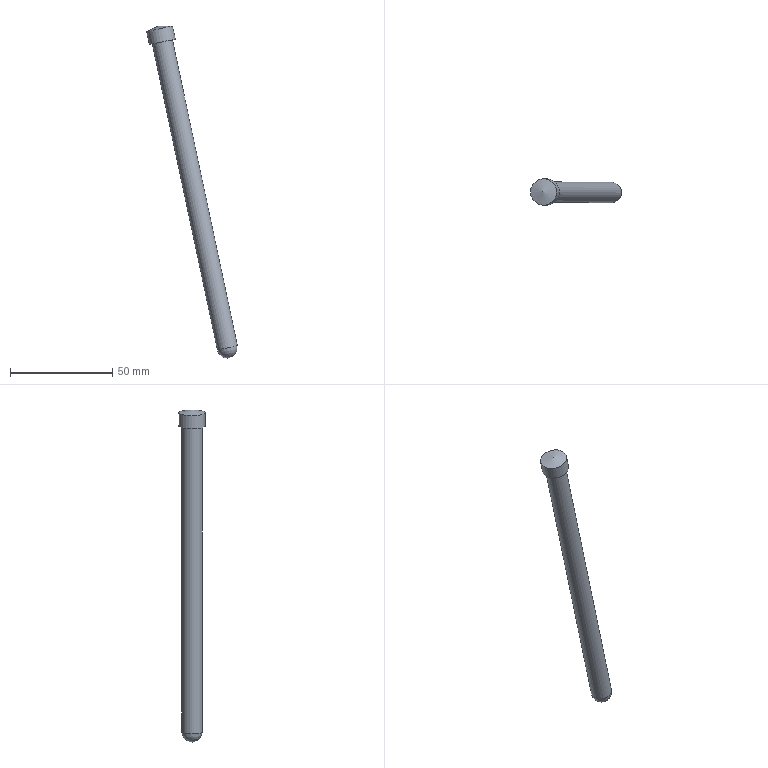Part | NX | features solid 2 | 1 solid | 5 faces | box 44.588 x 13 x 162.687 mm | volume 13234 mm3 | cylinder 2 | plane 1 | sphere 1 | cone 1 | commonest cylinder face diameters 10 x1 13 x1
STEP:
#1=CARTESIAN_POINT('',(112.348,-51.5,131.635));
#2=VERTEX_POINT('',#1);
#3=CARTESIAN_POINT('',(117.239,-51.5,132.675));
#4=DIRECTION('',(0.2079,0.,-0.9781));
#5=DIRECTION('',(-0.9781,0.,-0.2079));
#6=AXIS2_PLACEMENT_3D('',#3,#4,#5);
#7=CIRCLE('',#6,5.);
#8=EDGE_CURVE('',#2,#2,#7,.T.);
#9=ORIENTED_EDGE('',*,*,#8,.F.);
#10=EDGE_LOOP('',(#9));
#11=FACE_BOUND('',#10,.T.);
#12=CARTESIAN_POINT('',(110.881,-51.5,131.323));
#13=VERTEX_POINT('',#12);
#14=CARTESIAN_POINT('',(117.239,-51.5,132.675));
#15=DIRECTION('',(-0.2079,0.,0.9781));
#16=DIRECTION('',(-0.9781,0.,-0.2079));
#17=AXIS2_PLACEMENT_3D('',#14,#15,#16);
#18=CIRCLE('',#17,6.5);
#19=EDGE_CURVE('',#13,#13,#18,.T.);
#20=ORIENTED_EDGE('',*,*,#19,.F.);
#21=EDGE_LOOP('',(#20));
#22=FACE_BOUND('',#21,.T.);
#23=CARTESIAN_POINT('',(117.239,-51.5,132.675));
#24=DIRECTION('',(0.2079,0.,-0.9781));
#25=DIRECTION('',(-0.9781,0.,-0.2079));
#26=AXIS2_PLACEMENT_3D('',#23,#24,#25);
#27=PLANE('',#26);
#28=ADVANCED_FACE('',(#11,#22),#27,.T.);
#29=ORIENTED_EDGE('',*,*,#19,.T.);
#30=EDGE_LOOP('',(#29));
#31=FACE_BOUND('',#30,.T.);
#32=CARTESIAN_POINT('',(109.505,-51.5,137.797));
#33=VERTEX_POINT('',#32);
#34=CARTESIAN_POINT('',(115.863,-51.5,139.149));
#35=DIRECTION('',(0.2079,0.,-0.9781));
#36=DIRECTION('',(-0.9781,0.,-0.2079));
#37=AXIS2_PLACEMENT_3D('',#34,#35,#36);
#38=CIRCLE('',#37,6.5);
#39=EDGE_CURVE('',#33,#33,#38,.T.);
#40=ORIENTED_EDGE('',*,*,#39,.T.);
#41=EDGE_LOOP('',(#40));
#42=FACE_BOUND('',#41,.T.);
#43=CARTESIAN_POINT('',(115.863,-51.5,139.149));
#44=DIRECTION('',(0.2079,0.,-0.9781));
#45=DIRECTION('',(-0.9781,0.,-0.2079));
#46=AXIS2_PLACEMENT_3D('',#43,#44,#45);
#47=CYLINDRICAL_SURFACE('',#46,6.5);
#48=ADVANCED_FACE('',(#31,#42),#47,.T.);
#49=CARTESIAN_POINT('',(144.202,-51.5,-18.226));
#50=VERTEX_POINT('',#49);
#51=CARTESIAN_POINT('',(149.093,-51.5,-17.187));
#52=DIRECTION('',(0.2079,0.,-0.9781));
#53=DIRECTION('',(-0.9781,0.,-0.2079));
#54=AXIS2_PLACEMENT_3D('',#51,#52,#53);
#55=CIRCLE('',#54,5.);
#56=EDGE_CURVE('',#50,#50,#55,.T.);
#57=ORIENTED_EDGE('',*,*,#56,.F.);
#58=EDGE_LOOP('',(#57));
#59=FACE_BOUND('',#58,.T.);
#60=ORIENTED_EDGE('',*,*,#8,.T.);
#61=EDGE_LOOP('',(#60));
#62=FACE_BOUND('',#61,.T.);
#63=CARTESIAN_POINT('',(117.239,-51.5,132.675));
#64=DIRECTION('',(0.2079,0.,-0.9781));
#65=DIRECTION('',(-0.9781,0.,-0.2079));
#66=AXIS2_PLACEMENT_3D('',#63,#64,#65);
#67=CYLINDRICAL_SURFACE('',#66,5.);
#68=ADVANCED_FACE('',(#59,#62),#67,.T.);
#69=ORIENTED_EDGE('',*,*,#56,.T.);
#70=EDGE_LOOP('',(#69));
#71=FACE_BOUND('',#70,.T.);
#72=CARTESIAN_POINT('',(149.093,-51.5,-17.187));
#73=DIRECTION('',(0.2079,0.,-0.9781));
#74=DIRECTION('',(-0.9781,0.,-0.2079));
#75=AXIS2_PLACEMENT_3D('',#72,#73,#74);
#76=SPHERICAL_SURFACE('',#75,5.);
#77=ADVANCED_FACE('',(#71),#76,.T.);
#78=ORIENTED_EDGE('',*,*,#39,.F.);
#79=EDGE_LOOP('',(#78));
#80=FACE_BOUND('',#79,.T.);
#81=CARTESIAN_POINT('',(115.575,-51.5,140.5));
#82=VERTEX_POINT('',#81);
#83=VERTEX_LOOP('',#82);
#84=FACE_BOUND('',#83,.T.);
#85=CARTESIAN_POINT('',(115.575,-51.5,140.5));
#86=DIRECTION('',(0.2079,0.,-0.9781));
#87=DIRECTION('',(-0.9781,0.,-0.2079));
#88=AXIS2_PLACEMENT_3D('',#85,#86,#87);
#89=CONICAL_SURFACE('',#88,0.,1.361);
#90=ADVANCED_FACE('',(#80,#84),#89,.T.);
#91=CLOSED_SHELL('',(#28,#48,#68,#77,#90));
#92=MANIFOLD_SOLID_BREP('',#91);
#93=(LENGTH_UNIT()NAMED_UNIT(*)SI_UNIT(.MILLI.,.METRE.));
#94=UNCERTAINTY_MEASURE_WITH_UNIT(LENGTH_MEASURE(0.00001),#93,'','');
#95=(NAMED_UNIT(*)PLANE_ANGLE_UNIT()SI_UNIT($,.RADIAN.));
#96=(NAMED_UNIT(*)SI_UNIT($,.STERADIAN.)SOLID_ANGLE_UNIT());
#97=(GEOMETRIC_REPRESENTATION_CONTEXT(3)GLOBAL_UNCERTAINTY_ASSIGNED_CONTEXT((#94))GLOBAL_UNIT_ASSIGNED_CONTEXT((#93,#95,#96))REPRESENTATION_CONTEXT('',''));
#98=ADVANCED_BREP_SHAPE_REPRESENTATION('',(#92),#97);